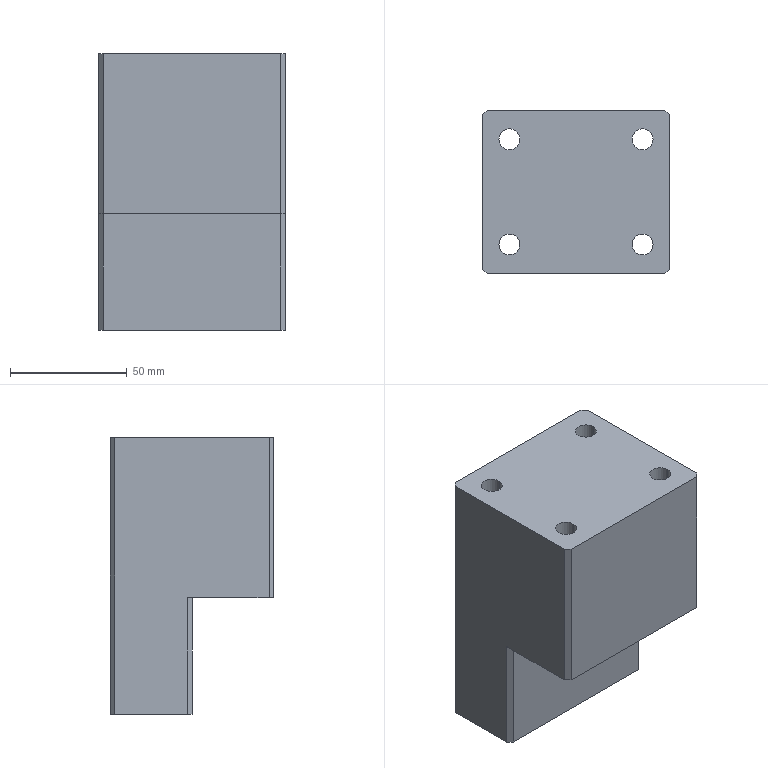Part | SolidWorks | features Cut 3, HoleWzd 2, Chamfer 1, Extrusion 1 | 1 solid | 46 faces | box 80 x 70 x 118.5 mm | volume 471238 mm3 | cylinder 22 | plane 18 | cone 6 | commonest cylinder face diameters 9 x8 14 x8 6.8 x4 14.5 x2
STEP:
#1=CARTESIAN_POINT('',(55.,50.25,6.6));
#2=VERTEX_POINT('',#1);
#3=CARTESIAN_POINT('',(55.,50.25,13.4));
#4=VERTEX_POINT('',#3);
#5=CARTESIAN_POINT('',(55.,50.25,10.));
#6=DIRECTION('',(0.,1.,0.));
#7=DIRECTION('',(0.,0.,1.));
#8=AXIS2_PLACEMENT_3D('',#5,#6,#7);
#9=CIRCLE('',#8,3.4);
#10=EDGE_CURVE('',#2,#4,#9,.T.);
#11=ORIENTED_EDGE('',*,*,#10,.F.);
#12=CARTESIAN_POINT('',(55.,70.,6.6));
#13=VERTEX_POINT('',#12);
#14=CARTESIAN_POINT('',(55.,70.,6.6));
#15=DIRECTION('',(0.,1.,0.));
#16=VECTOR('',#15,1000.);
#17=LINE('',#14,#16);
#18=EDGE_CURVE('',#2,#13,#17,.T.);
#19=ORIENTED_EDGE('',*,*,#18,.T.);
#20=CARTESIAN_POINT('',(55.,70.,13.4));
#21=VERTEX_POINT('',#20);
#22=CARTESIAN_POINT('',(55.,70.,10.));
#23=DIRECTION('',(0.,1.,0.));
#24=DIRECTION('',(0.,0.,1.));
#25=AXIS2_PLACEMENT_3D('',#22,#23,#24);
#26=CIRCLE('',#25,3.4);
#27=EDGE_CURVE('',#13,#21,#26,.T.);
#28=ORIENTED_EDGE('',*,*,#27,.T.);
#29=CARTESIAN_POINT('',(55.,70.,13.4));
#30=DIRECTION('',(0.,1.,0.));
#31=VECTOR('',#30,1000.);
#32=LINE('',#29,#31);
#33=EDGE_CURVE('',#4,#21,#32,.T.);
#34=ORIENTED_EDGE('',*,*,#33,.F.);
#35=EDGE_LOOP('',(#11,#19,#28,#34));
#36=FACE_OUTER_BOUND('',#35,.T.);
#37=CARTESIAN_POINT('',(55.,70.,10.));
#38=DIRECTION('',(0.,1.,0.));
#39=DIRECTION('',(0.,0.,1.));
#40=AXIS2_PLACEMENT_3D('',#37,#38,#39);
#41=CYLINDRICAL_SURFACE('',#40,3.4);
#42=ADVANCED_FACE('',(#36),#41,.F.);
#43=CARTESIAN_POINT('',(55.,48.207,10.));
#44=VERTEX_POINT('',#43);
#45=CARTESIAN_POINT('',(55.,50.25,13.4));
#46=DIRECTION('',(0.,0.515,0.8572));
#47=VECTOR('',#46,1000.);
#48=LINE('',#45,#47);
#49=EDGE_CURVE('',#44,#4,#48,.T.);
#50=ORIENTED_EDGE('',*,*,#49,.F.);
#51=CARTESIAN_POINT('',(55.,50.25,6.6));
#52=DIRECTION('',(0.,0.515,-0.8572));
#53=VECTOR('',#52,1000.);
#54=LINE('',#51,#53);
#55=EDGE_CURVE('',#44,#2,#54,.T.);
#56=ORIENTED_EDGE('',*,*,#55,.T.);
#57=ORIENTED_EDGE('',*,*,#10,.T.);
#58=EDGE_LOOP('',(#50,#56,#57));
#59=FACE_OUTER_BOUND('',#58,.T.);
#60=CARTESIAN_POINT('',(55.,50.25,10.));
#61=DIRECTION('',(0.,1.,0.));
#62=DIRECTION('',(0.,0.,1.));
#63=AXIS2_PLACEMENT_3D('',#60,#61,#62);
#64=CONICAL_SURFACE('',#63,3.4,1.03);
#65=ADVANCED_FACE('',(#59),#64,.F.);
#66=CARTESIAN_POINT('',(25.,50.25,6.6));
#67=VERTEX_POINT('',#66);
#68=CARTESIAN_POINT('',(25.,50.25,13.4));
#69=VERTEX_POINT('',#68);
#70=CARTESIAN_POINT('',(25.,50.25,10.));
#71=DIRECTION('',(0.,1.,0.));
#72=DIRECTION('',(0.,0.,1.));
#73=AXIS2_PLACEMENT_3D('',#70,#71,#72);
#74=CIRCLE('',#73,3.4);
#75=EDGE_CURVE('',#67,#69,#74,.T.);
#76=ORIENTED_EDGE('',*,*,#75,.F.);
#77=CARTESIAN_POINT('',(25.,70.,6.6));
#78=VERTEX_POINT('',#77);
#79=CARTESIAN_POINT('',(25.,70.,6.6));
#80=DIRECTION('',(0.,1.,0.));
#81=VECTOR('',#80,1000.);
#82=LINE('',#79,#81);
#83=EDGE_CURVE('',#67,#78,#82,.T.);
#84=ORIENTED_EDGE('',*,*,#83,.T.);
#85=CARTESIAN_POINT('',(25.,70.,13.4));
#86=VERTEX_POINT('',#85);
#87=CARTESIAN_POINT('',(25.,70.,10.));
#88=DIRECTION('',(0.,1.,0.));
#89=DIRECTION('',(0.,0.,1.));
#90=AXIS2_PLACEMENT_3D('',#87,#88,#89);
#91=CIRCLE('',#90,3.4);
#92=EDGE_CURVE('',#78,#86,#91,.T.);
#93=ORIENTED_EDGE('',*,*,#92,.T.);
#94=CARTESIAN_POINT('',(25.,70.,13.4));
#95=DIRECTION('',(0.,1.,0.));
#96=VECTOR('',#95,1000.);
#97=LINE('',#94,#96);
#98=EDGE_CURVE('',#69,#86,#97,.T.);
#99=ORIENTED_EDGE('',*,*,#98,.F.);
#100=EDGE_LOOP('',(#76,#84,#93,#99));
#101=FACE_OUTER_BOUND('',#100,.T.);
#102=CARTESIAN_POINT('',(25.,70.,10.));
#103=DIRECTION('',(0.,1.,0.));
#104=DIRECTION('',(0.,0.,1.));
#105=AXIS2_PLACEMENT_3D('',#102,#103,#104);
#106=CYLINDRICAL_SURFACE('',#105,3.4);
#107=ADVANCED_FACE('',(#101),#106,.F.);
#108=CARTESIAN_POINT('',(25.,48.207,10.));
#109=VERTEX_POINT('',#108);
#110=CARTESIAN_POINT('',(25.,50.25,13.4));
#111=DIRECTION('',(0.,0.515,0.8572));
#112=VECTOR('',#111,1000.);
#113=LINE('',#110,#112);
#114=EDGE_CURVE('',#109,#69,#113,.T.);
#115=ORIENTED_EDGE('',*,*,#114,.F.);
#116=CARTESIAN_POINT('',(25.,50.25,6.6));
#117=DIRECTION('',(0.,0.515,-0.8572));
#118=VECTOR('',#117,1000.);
#119=LINE('',#116,#118);
#120=EDGE_CURVE('',#109,#67,#119,.T.);
#121=ORIENTED_EDGE('',*,*,#120,.T.);
#122=ORIENTED_EDGE('',*,*,#75,.T.);
#123=EDGE_LOOP('',(#115,#121,#122));
#124=FACE_OUTER_BOUND('',#123,.T.);
#125=CARTESIAN_POINT('',(25.,50.25,10.));
#126=DIRECTION('',(0.,1.,0.));
#127=DIRECTION('',(0.,0.,1.));
#128=AXIS2_PLACEMENT_3D('',#125,#126,#127);
#129=CONICAL_SURFACE('',#128,3.4,1.03);
#130=ADVANCED_FACE('',(#124),#129,.F.);
#131=CARTESIAN_POINT('',(40.,33.5,90.25));
#132=VERTEX_POINT('',#131);
#133=CARTESIAN_POINT('',(40.,33.5,104.75));
#134=VERTEX_POINT('',#133);
#135=CARTESIAN_POINT('',(40.,33.5,97.5));
#136=DIRECTION('',(0.,1.,0.));
#137=DIRECTION('',(0.,0.,1.));
#138=AXIS2_PLACEMENT_3D('',#135,#136,#137);
#139=CIRCLE('',#138,7.25);
#140=EDGE_CURVE('',#132,#134,#139,.T.);
#141=ORIENTED_EDGE('',*,*,#140,.F.);
#142=CARTESIAN_POINT('',(40.,70.,90.25));
#143=VERTEX_POINT('',#142);
#144=CARTESIAN_POINT('',(40.,70.,90.25));
#145=DIRECTION('',(0.,1.,0.));
#146=VECTOR('',#145,1000.);
#147=LINE('',#144,#146);
#148=EDGE_CURVE('',#132,#143,#147,.T.);
#149=ORIENTED_EDGE('',*,*,#148,.T.);
#150=CARTESIAN_POINT('',(40.,70.,104.75));
#151=VERTEX_POINT('',#150);
#152=CARTESIAN_POINT('',(40.,70.,97.5));
#153=DIRECTION('',(0.,1.,0.));
#154=DIRECTION('',(0.,0.,1.));
#155=AXIS2_PLACEMENT_3D('',#152,#153,#154);
#156=CIRCLE('',#155,7.25);
#157=EDGE_CURVE('',#143,#151,#156,.T.);
#158=ORIENTED_EDGE('',*,*,#157,.T.);
#159=CARTESIAN_POINT('',(40.,70.,104.75));
#160=DIRECTION('',(0.,1.,0.));
#161=VECTOR('',#160,1000.);
#162=LINE('',#159,#161);
#163=EDGE_CURVE('',#134,#151,#162,.T.);
#164=ORIENTED_EDGE('',*,*,#163,.F.);
#165=EDGE_LOOP('',(#141,#149,#158,#164));
#166=FACE_OUTER_BOUND('',#165,.T.);
#167=CARTESIAN_POINT('',(40.,70.,97.5));
#168=DIRECTION('',(0.,1.,0.));
#169=DIRECTION('',(0.,0.,1.));
#170=AXIS2_PLACEMENT_3D('',#167,#168,#169);
#171=CYLINDRICAL_SURFACE('',#170,7.25);
#172=ADVANCED_FACE('',(#166),#171,.F.);
#173=CARTESIAN_POINT('',(40.,29.144,97.5));
#174=VERTEX_POINT('',#173);
#175=CARTESIAN_POINT('',(40.,33.5,104.75));
#176=DIRECTION('',(0.,0.515,0.8572));
#177=VECTOR('',#176,1000.);
#178=LINE('',#175,#177);
#179=EDGE_CURVE('',#174,#134,#178,.T.);
#180=ORIENTED_EDGE('',*,*,#179,.F.);
#181=CARTESIAN_POINT('',(40.,33.5,90.25));
#182=DIRECTION('',(0.,0.515,-0.8572));
#183=VECTOR('',#182,1000.);
#184=LINE('',#181,#183);
#185=EDGE_CURVE('',#174,#132,#184,.T.);
#186=ORIENTED_EDGE('',*,*,#185,.T.);
#187=ORIENTED_EDGE('',*,*,#140,.T.);
#188=EDGE_LOOP('',(#180,#186,#187));
#189=FACE_OUTER_BOUND('',#188,.T.);
#190=CARTESIAN_POINT('',(40.,33.5,97.5));
#191=DIRECTION('',(0.,1.,0.));
#192=DIRECTION('',(0.,0.,1.));
#193=AXIS2_PLACEMENT_3D('',#190,#191,#192);
#194=CONICAL_SURFACE('',#193,7.25,1.03);
#195=ADVANCED_FACE('',(#189),#194,.F.);
#196=CARTESIAN_POINT('',(73.,12.5,118.5));
#197=VERTEX_POINT('',#196);
#198=CARTESIAN_POINT('',(64.,12.5,118.5));
#199=VERTEX_POINT('',#198);
#200=CARTESIAN_POINT('',(68.5,12.5,118.5));
#201=DIRECTION('',(0.,0.,-1.));
#202=DIRECTION('',(-1.,0.,0.));
#203=AXIS2_PLACEMENT_3D('',#200,#201,#202);
#204=CIRCLE('',#203,4.5);
#205=EDGE_CURVE('',#197,#199,#204,.T.);
#206=ORIENTED_EDGE('',*,*,#205,.F.);
#207=CARTESIAN_POINT('',(73.,12.5,80.));
#208=VERTEX_POINT('',#207);
#209=CARTESIAN_POINT('',(73.,12.5,118.5));
#210=DIRECTION('',(0.,0.,-1.));
#211=VECTOR('',#210,1000.);
#212=LINE('',#209,#211);
#213=EDGE_CURVE('',#197,#208,#212,.T.);
#214=ORIENTED_EDGE('',*,*,#213,.T.);
#215=CARTESIAN_POINT('',(64.,12.5,80.));
#216=VERTEX_POINT('',#215);
#217=CARTESIAN_POINT('',(68.5,12.5,80.));
#218=DIRECTION('',(0.,0.,-1.));
#219=DIRECTION('',(-1.,0.,0.));
#220=AXIS2_PLACEMENT_3D('',#217,#218,#219);
#221=CIRCLE('',#220,4.5);
#222=EDGE_CURVE('',#208,#216,#221,.T.);
#223=ORIENTED_EDGE('',*,*,#222,.T.);
#224=CARTESIAN_POINT('',(64.,12.5,118.5));
#225=DIRECTION('',(0.,0.,-1.));
#226=VECTOR('',#225,1000.);
#227=LINE('',#224,#226);
#228=EDGE_CURVE('',#199,#216,#227,.T.);
#229=ORIENTED_EDGE('',*,*,#228,.F.);
#230=EDGE_LOOP('',(#206,#214,#223,#229));
#231=FACE_OUTER_BOUND('',#230,.T.);
#232=CARTESIAN_POINT('',(68.5,12.5,118.5));
#233=DIRECTION('',(0.,0.,-1.));
#234=DIRECTION('',(-1.,0.,0.));
#235=AXIS2_PLACEMENT_3D('',#232,#233,#234);
#236=CYLINDRICAL_SURFACE('',#235,4.5);
#237=ADVANCED_FACE('',(#231),#236,.F.);
#238=CARTESIAN_POINT('',(16.,12.5,118.5));
#239=VERTEX_POINT('',#238);
#240=CARTESIAN_POINT('',(7.,12.5,118.5));
#241=VERTEX_POINT('',#240);
#242=CARTESIAN_POINT('',(11.5,12.5,118.5));
#243=DIRECTION('',(0.,0.,-1.));
#244=DIRECTION('',(-1.,0.,0.));
#245=AXIS2_PLACEMENT_3D('',#242,#243,#244);
#246=CIRCLE('',#245,4.5);
#247=EDGE_CURVE('',#239,#241,#246,.T.);
#248=ORIENTED_EDGE('',*,*,#247,.F.);
#249=CARTESIAN_POINT('',(16.,12.5,80.));
#250=VERTEX_POINT('',#249);
#251=CARTESIAN_POINT('',(16.,12.5,118.5));
#252=DIRECTION('',(0.,0.,-1.));
#253=VECTOR('',#252,1000.);
#254=LINE('',#251,#253);
#255=EDGE_CURVE('',#239,#250,#254,.T.);
#256=ORIENTED_EDGE('',*,*,#255,.T.);
#257=CARTESIAN_POINT('',(7.,12.5,80.));
#258=VERTEX_POINT('',#257);
#259=CARTESIAN_POINT('',(11.5,12.5,80.));
#260=DIRECTION('',(0.,0.,-1.));
#261=DIRECTION('',(-1.,0.,0.));
#262=AXIS2_PLACEMENT_3D('',#259,#260,#261);
#263=CIRCLE('',#262,4.5);
#264=EDGE_CURVE('',#250,#258,#263,.T.);
#265=ORIENTED_EDGE('',*,*,#264,.T.);
#266=CARTESIAN_POINT('',(7.,12.5,118.5));
#267=DIRECTION('',(0.,0.,-1.));
#268=VECTOR('',#267,1000.);
#269=LINE('',#266,#268);
#270=EDGE_CURVE('',#241,#258,#269,.T.);
#271=ORIENTED_EDGE('',*,*,#270,.F.);
#272=EDGE_LOOP('',(#248,#256,#265,#271));
#273=FACE_OUTER_BOUND('',#272,.T.);
#274=CARTESIAN_POINT('',(11.5,12.5,118.5));
#275=DIRECTION('',(0.,0.,-1.));
#276=DIRECTION('',(-1.,0.,0.));
#277=AXIS2_PLACEMENT_3D('',#274,#275,#276);
#278=CYLINDRICAL_SURFACE('',#277,4.5);
#279=ADVANCED_FACE('',(#273),#278,.F.);
#280=CARTESIAN_POINT('',(16.,57.5,118.5));
#281=VERTEX_POINT('',#280);
#282=CARTESIAN_POINT('',(7.,57.5,118.5));
#283=VERTEX_POINT('',#282);
#284=CARTESIAN_POINT('',(11.5,57.5,118.5));
#285=DIRECTION('',(0.,0.,-1.));
#286=DIRECTION('',(-1.,0.,0.));
#287=AXIS2_PLACEMENT_3D('',#284,#285,#286);
#288=CIRCLE('',#287,4.5);
#289=EDGE_CURVE('',#281,#283,#288,.T.);
#290=ORIENTED_EDGE('',*,*,#289,.F.);
#291=CARTESIAN_POINT('',(16.,57.5,80.));
#292=VERTEX_POINT('',#291);
#293=CARTESIAN_POINT('',(16.,57.5,118.5));
#294=DIRECTION('',(0.,0.,-1.));
#295=VECTOR('',#294,1000.);
#296=LINE('',#293,#295);
#297=EDGE_CURVE('',#281,#292,#296,.T.);
#298=ORIENTED_EDGE('',*,*,#297,.T.);
#299=CARTESIAN_POINT('',(7.,57.5,80.));
#300=VERTEX_POINT('',#299);
#301=CARTESIAN_POINT('',(11.5,57.5,80.));
#302=DIRECTION('',(0.,0.,-1.));
#303=DIRECTION('',(-1.,0.,0.));
#304=AXIS2_PLACEMENT_3D('',#301,#302,#303);
#305=CIRCLE('',#304,4.5);
#306=EDGE_CURVE('',#292,#300,#305,.T.);
#307=ORIENTED_EDGE('',*,*,#306,.T.);
#308=CARTESIAN_POINT('',(7.,57.5,118.5));
#309=DIRECTION('',(0.,0.,-1.));
#310=VECTOR('',#309,1000.);
#311=LINE('',#308,#310);
#312=EDGE_CURVE('',#283,#300,#311,.T.);
#313=ORIENTED_EDGE('',*,*,#312,.F.);
#314=EDGE_LOOP('',(#290,#298,#307,#313));
#315=FACE_OUTER_BOUND('',#314,.T.);
#316=CARTESIAN_POINT('',(11.5,57.5,118.5));
#317=DIRECTION('',(0.,0.,-1.));
#318=DIRECTION('',(-1.,0.,0.));
#319=AXIS2_PLACEMENT_3D('',#316,#317,#318);
#320=CYLINDRICAL_SURFACE('',#319,4.5);
#321=ADVANCED_FACE('',(#315),#320,.F.);
#322=CARTESIAN_POINT('',(73.,57.5,118.5));
#323=VERTEX_POINT('',#322);
#324=CARTESIAN_POINT('',(64.,57.5,118.5));
#325=VERTEX_POINT('',#324);
#326=CARTESIAN_POINT('',(68.5,57.5,118.5));
#327=DIRECTION('',(0.,0.,-1.));
#328=DIRECTION('',(-1.,0.,0.));
#329=AXIS2_PLACEMENT_3D('',#326,#327,#328);
#330=CIRCLE('',#329,4.5);
#331=EDGE_CURVE('',#323,#325,#330,.T.);
#332=ORIENTED_EDGE('',*,*,#331,.F.);
#333=CARTESIAN_POINT('',(73.,57.5,80.));
#334=VERTEX_POINT('',#333);
#335=CARTESIAN_POINT('',(73.,57.5,118.5));
#336=DIRECTION('',(0.,0.,-1.));
#337=VECTOR('',#336,1000.);
#338=LINE('',#335,#337);
#339=EDGE_CURVE('',#323,#334,#338,.T.);
#340=ORIENTED_EDGE('',*,*,#339,.T.);
#341=CARTESIAN_POINT('',(64.,57.5,80.));
#342=VERTEX_POINT('',#341);
#343=CARTESIAN_POINT('',(68.5,57.5,80.));
#344=DIRECTION('',(0.,0.,-1.));
#345=DIRECTION('',(-1.,0.,0.));
#346=AXIS2_PLACEMENT_3D('',#343,#344,#345);
#347=CIRCLE('',#346,4.5);
#348=EDGE_CURVE('',#334,#342,#347,.T.);
#349=ORIENTED_EDGE('',*,*,#348,.T.);
#350=CARTESIAN_POINT('',(64.,57.5,118.5));
#351=DIRECTION('',(0.,0.,-1.));
#352=VECTOR('',#351,1000.);
#353=LINE('',#350,#352);
#354=EDGE_CURVE('',#325,#342,#353,.T.);
#355=ORIENTED_EDGE('',*,*,#354,.F.);
#356=EDGE_LOOP('',(#332,#340,#349,#355));
#357=FACE_OUTER_BOUND('',#356,.T.);
#358=CARTESIAN_POINT('',(68.5,57.5,118.5));
#359=DIRECTION('',(0.,0.,-1.));
#360=DIRECTION('',(-1.,0.,0.));
#361=AXIS2_PLACEMENT_3D('',#358,#359,#360);
#362=CYLINDRICAL_SURFACE('',#361,4.5);
#363=ADVANCED_FACE('',(#357),#362,.F.);
#364=CARTESIAN_POINT('',(75.5,12.5,80.));
#365=VERTEX_POINT('',#364);
#366=CARTESIAN_POINT('',(61.5,12.5,80.));
#367=VERTEX_POINT('',#366);
#368=CARTESIAN_POINT('',(68.5,12.5,80.));
#369=DIRECTION('',(0.,0.,-1.));
#370=DIRECTION('',(-1.,0.,0.));
#371=AXIS2_PLACEMENT_3D('',#368,#369,#370);
#372=CIRCLE('',#371,7.);
#373=EDGE_CURVE('',#365,#367,#372,.T.);
#374=ORIENTED_EDGE('',*,*,#373,.F.);
#375=CARTESIAN_POINT('',(75.5,12.5,50.));
#376=VERTEX_POINT('',#375);
#377=CARTESIAN_POINT('',(75.5,12.5,80.));
#378=DIRECTION('',(0.,0.,-1.));
#379=VECTOR('',#378,1000.);
#380=LINE('',#377,#379);
#381=EDGE_CURVE('',#365,#376,#380,.T.);
#382=ORIENTED_EDGE('',*,*,#381,.T.);
#383=CARTESIAN_POINT('',(61.5,12.5,50.));
#384=VERTEX_POINT('',#383);
#385=CARTESIAN_POINT('',(68.5,12.5,50.));
#386=DIRECTION('',(0.,0.,-1.));
#387=DIRECTION('',(1.,0.,0.));
#388=AXIS2_PLACEMENT_3D('',#385,#386,#387);
#389=CIRCLE('',#388,7.);
#390=EDGE_CURVE('',#376,#384,#389,.T.);
#391=ORIENTED_EDGE('',*,*,#390,.T.);
#392=CARTESIAN_POINT('',(61.5,12.5,80.));
#393=DIRECTION('',(0.,0.,-1.));
#394=VECTOR('',#393,1000.);
#395=LINE('',#392,#394);
#396=EDGE_CURVE('',#367,#384,#395,.T.);
#397=ORIENTED_EDGE('',*,*,#396,.F.);
#398=EDGE_LOOP('',(#374,#382,#391,#397));
#399=FACE_OUTER_BOUND('',#398,.T.);
#400=CARTESIAN_POINT('',(68.5,12.5,80.));
#401=DIRECTION('',(0.,0.,-1.));
#402=DIRECTION('',(-1.,0.,0.));
#403=AXIS2_PLACEMENT_3D('',#400,#401,#402);
#404=CYLINDRICAL_SURFACE('',#403,7.);
#405=ADVANCED_FACE('',(#399),#404,.F.);
#406=CARTESIAN_POINT('',(75.5,57.5,80.));
#407=VERTEX_POINT('',#406);
#408=CARTESIAN_POINT('',(61.5,57.5,80.));
#409=VERTEX_POINT('',#408);
#410=CARTESIAN_POINT('',(68.5,57.5,80.));
#411=DIRECTION('',(0.,0.,-1.));
#412=DIRECTION('',(-1.,0.,0.));
#413=AXIS2_PLACEMENT_3D('',#410,#411,#412);
#414=CIRCLE('',#413,7.);
#415=EDGE_CURVE('',#407,#409,#414,.T.);
#416=ORIENTED_EDGE('',*,*,#415,.F.);
#417=CARTESIAN_POINT('',(75.5,57.5,0.));
#418=VERTEX_POINT('',#417);
#419=CARTESIAN_POINT('',(75.5,57.5,80.));
#420=DIRECTION('',(0.,0.,-1.));
#421=VECTOR('',#420,1000.);
#422=LINE('',#419,#421);
#423=EDGE_CURVE('',#407,#418,#422,.T.);
#424=ORIENTED_EDGE('',*,*,#423,.T.);
#425=CARTESIAN_POINT('',(61.5,57.5,0.));
#426=VERTEX_POINT('',#425);
#427=CARTESIAN_POINT('',(68.5,57.5,0.));
#428=DIRECTION('',(0.,0.,-1.));
#429=DIRECTION('',(-1.,0.,0.));
#430=AXIS2_PLACEMENT_3D('',#427,#428,#429);
#431=CIRCLE('',#430,7.);
#432=EDGE_CURVE('',#418,#426,#431,.T.);
#433=ORIENTED_EDGE('',*,*,#432,.T.);
#434=CARTESIAN_POINT('',(61.5,57.5,80.));
#435=DIRECTION('',(0.,0.,-1.));
#436=VECTOR('',#435,1000.);
#437=LINE('',#434,#436);
#438=EDGE_CURVE('',#409,#426,#437,.T.);
#439=ORIENTED_EDGE('',*,*,#438,.F.);
#440=EDGE_LOOP('',(#416,#424,#433,#439));
#441=FACE_OUTER_BOUND('',#440,.T.);
#442=CARTESIAN_POINT('',(68.5,57.5,80.));
#443=DIRECTION('',(0.,0.,-1.));
#444=DIRECTION('',(-1.,0.,0.));
#445=AXIS2_PLACEMENT_3D('',#442,#443,#444);
#446=CYLINDRICAL_SURFACE('',#445,7.);
#447=ADVANCED_FACE('',(#441),#446,.F.);
#448=CARTESIAN_POINT('',(18.5,12.5,80.));
#449=VERTEX_POINT('',#448);
#450=CARTESIAN_POINT('',(4.5,12.5,80.));
#451=VERTEX_POINT('',#450);
#452=CARTESIAN_POINT('',(11.5,12.5,80.));
#453=DIRECTION('',(0.,0.,-1.));
#454=DIRECTION('',(-1.,0.,0.));
#455=AXIS2_PLACEMENT_3D('',#452,#453,#454);
#456=CIRCLE('',#455,7.);
#457=EDGE_CURVE('',#449,#451,#456,.T.);
#458=ORIENTED_EDGE('',*,*,#457,.F.);
#459=CARTESIAN_POINT('',(18.5,12.5,50.));
#460=VERTEX_POINT('',#459);
#461=CARTESIAN_POINT('',(18.5,12.5,80.));
#462=DIRECTION('',(0.,0.,-1.));
#463=VECTOR('',#462,1000.);
#464=LINE('',#461,#463);
#465=EDGE_CURVE('',#449,#460,#464,.T.);
#466=ORIENTED_EDGE('',*,*,#465,.T.);
#467=CARTESIAN_POINT('',(4.5,12.5,50.));
#468=VERTEX_POINT('',#467);
#469=CARTESIAN_POINT('',(11.5,12.5,50.));
#470=DIRECTION('',(0.,0.,-1.));
#471=DIRECTION('',(1.,0.,0.));
#472=AXIS2_PLACEMENT_3D('',#469,#470,#471);
#473=CIRCLE('',#472,7.);
#474=EDGE_CURVE('',#460,#468,#473,.T.);
#475=ORIENTED_EDGE('',*,*,#474,.T.);
#476=CARTESIAN_POINT('',(4.5,12.5,80.));
#477=DIRECTION('',(0.,0.,-1.));
#478=VECTOR('',#477,1000.);
#479=LINE('',#476,#478);
#480=EDGE_CURVE('',#451,#468,#479,.T.);
#481=ORIENTED_EDGE('',*,*,#480,.F.);
#482=EDGE_LOOP('',(#458,#466,#475,#481));
#483=FACE_OUTER_BOUND('',#482,.T.);
#484=CARTESIAN_POINT('',(11.5,12.5,80.));
#485=DIRECTION('',(0.,0.,-1.));
#486=DIRECTION('',(-1.,0.,0.));
#487=AXIS2_PLACEMENT_3D('',#484,#485,#486);
#488=CYLINDRICAL_SURFACE('',#487,7.);
#489=ADVANCED_FACE('',(#483),#488,.F.);
#490=CARTESIAN_POINT('',(18.5,57.5,80.));
#491=VERTEX_POINT('',#490);
#492=CARTESIAN_POINT('',(4.5,57.5,80.));
#493=VERTEX_POINT('',#492);
#494=CARTESIAN_POINT('',(11.5,57.5,80.));
#495=DIRECTION('',(0.,0.,-1.));
#496=DIRECTION('',(-1.,0.,0.));
#497=AXIS2_PLACEMENT_3D('',#494,#495,#496);
#498=CIRCLE('',#497,7.);
#499=EDGE_CURVE('',#491,#493,#498,.T.);
#500=ORIENTED_EDGE('',*,*,#499,.F.);
#501=CARTESIAN_POINT('',(18.5,57.5,0.));
#502=VERTEX_POINT('',#501);
#503=CARTESIAN_POINT('',(18.5,57.5,80.));
#504=DIRECTION('',(0.,0.,-1.));
#505=VECTOR('',#504,1000.);
#506=LINE('',#503,#505);
#507=EDGE_CURVE('',#491,#502,#506,.T.);
#508=ORIENTED_EDGE('',*,*,#507,.T.);
#509=CARTESIAN_POINT('',(4.5,57.5,0.));
#510=VERTEX_POINT('',#509);
#511=CARTESIAN_POINT('',(11.5,57.5,0.));
#512=DIRECTION('',(0.,0.,-1.));
#513=DIRECTION('',(-1.,0.,0.));
#514=AXIS2_PLACEMENT_3D('',#511,#512,#513);
#515=CIRCLE('',#514,7.);
#516=EDGE_CURVE('',#502,#510,#515,.T.);
#517=ORIENTED_EDGE('',*,*,#516,.T.);
#518=CARTESIAN_POINT('',(4.5,57.5,80.));
#519=DIRECTION('',(0.,0.,-1.));
#520=VECTOR('',#519,1000.);
#521=LINE('',#518,#520);
#522=EDGE_CURVE('',#493,#510,#521,.T.);
#523=ORIENTED_EDGE('',*,*,#522,.F.);
#524=EDGE_LOOP('',(#500,#508,#517,#523));
#525=FACE_OUTER_BOUND('',#524,.T.);
#526=CARTESIAN_POINT('',(11.5,57.5,80.));
#527=DIRECTION('',(0.,0.,-1.));
#528=DIRECTION('',(-1.,0.,0.));
#529=AXIS2_PLACEMENT_3D('',#526,#527,#528);
#530=CYLINDRICAL_SURFACE('',#529,7.);
#531=ADVANCED_FACE('',(#525),#530,.F.);
#532=CARTESIAN_POINT('',(0.,68.,0.));
#533=VERTEX_POINT('',#532);
#534=CARTESIAN_POINT('',(0.,37.,0.));
#535=VERTEX_POINT('',#534);
#536=CARTESIAN_POINT('',(0.,0.,0.));
#537=DIRECTION('',(0.,-1.,0.));
#538=VECTOR('',#537,1000.);
#539=LINE('',#536,#538);
#540=EDGE_CURVE('',#533,#535,#539,.T.);
#541=ORIENTED_EDGE('',*,*,#540,.T.);
#542=CARTESIAN_POINT('',(0.,37.,50.));
#543=VERTEX_POINT('',#542);
#544=CARTESIAN_POINT('',(0.,37.,118.5));
#545=DIRECTION('',(0.,0.,1.));
#546=VECTOR('',#545,1000.);
#547=LINE('',#544,#546);
#548=EDGE_CURVE('',#535,#543,#547,.T.);
#549=ORIENTED_EDGE('',*,*,#548,.T.);
#550=CARTESIAN_POINT('',(0.,2.,50.));
#551=VERTEX_POINT('',#550);
#552=CARTESIAN_POINT('',(0.,0.,50.));
#553=DIRECTION('',(0.,1.,0.));
#554=VECTOR('',#553,1000.);
#555=LINE('',#552,#554);
#556=EDGE_CURVE('',#551,#543,#555,.T.);
#557=ORIENTED_EDGE('',*,*,#556,.F.);
#558=CARTESIAN_POINT('',(0.,2.,118.5));
#559=VERTEX_POINT('',#558);
#560=CARTESIAN_POINT('',(0.,2.,118.5));
#561=DIRECTION('',(0.,0.,1.));
#562=VECTOR('',#561,1000.);
#563=LINE('',#560,#562);
#564=EDGE_CURVE('',#551,#559,#563,.T.);
#565=ORIENTED_EDGE('',*,*,#564,.T.);
#566=CARTESIAN_POINT('',(0.,68.,118.5));
#567=VERTEX_POINT('',#566);
#568=CARTESIAN_POINT('',(0.,0.,118.5));
#569=DIRECTION('',(0.,-1.,0.));
#570=VECTOR('',#569,1000.);
#571=LINE('',#568,#570);
#572=EDGE_CURVE('',#567,#559,#571,.T.);
#573=ORIENTED_EDGE('',*,*,#572,.F.);
#574=CARTESIAN_POINT('',(0.,68.,118.5));
#575=DIRECTION('',(0.,0.,-1.));
#576=VECTOR('',#575,1000.);
#577=LINE('',#574,#576);
#578=EDGE_CURVE('',#567,#533,#577,.T.);
#579=ORIENTED_EDGE('',*,*,#578,.T.);
#580=EDGE_LOOP('',(#541,#549,#557,#565,#573,#579));
#581=FACE_OUTER_BOUND('',#580,.T.);
#582=CARTESIAN_POINT('',(0.,0.,118.5));
#583=DIRECTION('',(1.,0.,0.));
#584=DIRECTION('',(0.,1.,0.));
#585=AXIS2_PLACEMENT_3D('',#582,#583,#584);
#586=PLANE('',#585);
#587=ADVANCED_FACE('',(#581),#586,.F.);
#588=CARTESIAN_POINT('',(2.,0.,118.5));
#589=VERTEX_POINT('',#588);
#590=CARTESIAN_POINT('',(78.,0.,118.5));
#591=VERTEX_POINT('',#590);
#592=CARTESIAN_POINT('',(0.,0.,118.5));
#593=DIRECTION('',(1.,0.,0.));
#594=VECTOR('',#593,1000.);
#595=LINE('',#592,#594);
#596=EDGE_CURVE('',#589,#591,#595,.T.);
#597=ORIENTED_EDGE('',*,*,#596,.F.);
#598=CARTESIAN_POINT('',(2.,0.,50.));
#599=VERTEX_POINT('',#598);
#600=CARTESIAN_POINT('',(2.,0.,118.5));
#601=DIRECTION('',(0.,0.,-1.));
#602=VECTOR('',#601,1000.);
#603=LINE('',#600,#602);
#604=EDGE_CURVE('',#589,#599,#603,.T.);
#605=ORIENTED_EDGE('',*,*,#604,.T.);
#606=CARTESIAN_POINT('',(78.,0.,50.));
#607=VERTEX_POINT('',#606);
#608=CARTESIAN_POINT('',(80.,0.,50.));
#609=DIRECTION('',(-1.,0.,0.));
#610=VECTOR('',#609,1000.);
#611=LINE('',#608,#610);
#612=EDGE_CURVE('',#607,#599,#611,.T.);
#613=ORIENTED_EDGE('',*,*,#612,.F.);
#614=CARTESIAN_POINT('',(78.,0.,118.5));
#615=DIRECTION('',(0.,0.,1.));
#616=VECTOR('',#615,1000.);
#617=LINE('',#614,#616);
#618=EDGE_CURVE('',#607,#591,#617,.T.);
#619=ORIENTED_EDGE('',*,*,#618,.T.);
#620=EDGE_LOOP('',(#597,#605,#613,#619));
#621=FACE_OUTER_BOUND('',#620,.T.);
#622=CARTESIAN_POINT('',(0.,0.,118.5));
#623=DIRECTION('',(0.,1.,0.));
#624=DIRECTION('',(0.,0.,1.));
#625=AXIS2_PLACEMENT_3D('',#622,#623,#624);
#626=PLANE('',#625);
#627=ADVANCED_FACE('',(#621),#626,.F.);
#628=CARTESIAN_POINT('',(80.,37.,50.));
#629=VERTEX_POINT('',#628);
#630=CARTESIAN_POINT('',(80.,2.,50.));
#631=VERTEX_POINT('',#630);
#632=CARTESIAN_POINT('',(80.,0.,50.));
#633=DIRECTION('',(0.,-1.,0.));
#634=VECTOR('',#633,1000.);
#635=LINE('',#632,#634);
#636=EDGE_CURVE('',#629,#631,#635,.T.);
#637=ORIENTED_EDGE('',*,*,#636,.F.);
#638=CARTESIAN_POINT('',(80.,37.,0.));
#639=VERTEX_POINT('',#638);
#640=CARTESIAN_POINT('',(80.,37.,118.5));
#641=DIRECTION('',(0.,0.,-1.));
#642=VECTOR('',#641,1000.);
#643=LINE('',#640,#642);
#644=EDGE_CURVE('',#629,#639,#643,.T.);
#645=ORIENTED_EDGE('',*,*,#644,.T.);
#646=CARTESIAN_POINT('',(80.,68.,0.));
#647=VERTEX_POINT('',#646);
#648=CARTESIAN_POINT('',(80.,0.,0.));
#649=DIRECTION('',(0.,1.,0.));
#650=VECTOR('',#649,1000.);
#651=LINE('',#648,#650);
#652=EDGE_CURVE('',#639,#647,#651,.T.);
#653=ORIENTED_EDGE('',*,*,#652,.T.);
#654=CARTESIAN_POINT('',(80.,68.,118.5));
#655=VERTEX_POINT('',#654);
#656=CARTESIAN_POINT('',(80.,68.,118.5));
#657=DIRECTION('',(0.,0.,1.));
#658=VECTOR('',#657,1000.);
#659=LINE('',#656,#658);
#660=EDGE_CURVE('',#647,#655,#659,.T.);
#661=ORIENTED_EDGE('',*,*,#660,.T.);
#662=CARTESIAN_POINT('',(80.,2.,118.5));
#663=VERTEX_POINT('',#662);
#664=CARTESIAN_POINT('',(80.,0.,118.5));
#665=DIRECTION('',(0.,1.,0.));
#666=VECTOR('',#665,1000.);
#667=LINE('',#664,#666);
#668=EDGE_CURVE('',#663,#655,#667,.T.);
#669=ORIENTED_EDGE('',*,*,#668,.F.);
#670=CARTESIAN_POINT('',(80.,2.,118.5));
#671=DIRECTION('',(0.,0.,-1.));
#672=VECTOR('',#671,1000.);
#673=LINE('',#670,#672);
#674=EDGE_CURVE('',#663,#631,#673,.T.);
#675=ORIENTED_EDGE('',*,*,#674,.T.);
#676=EDGE_LOOP('',(#637,#645,#653,#661,#669,#675));
#677=FACE_OUTER_BOUND('',#676,.T.);
#678=CARTESIAN_POINT('',(80.,0.,118.5));
#679=DIRECTION('',(-1.,0.,0.));
#680=DIRECTION('',(0.,-1.,0.));
#681=AXIS2_PLACEMENT_3D('',#678,#679,#680);
#682=PLANE('',#681);
#683=ADVANCED_FACE('',(#677),#682,.F.);
#684=CARTESIAN_POINT('',(55.,70.,10.));
#685=DIRECTION('',(0.,1.,0.));
#686=DIRECTION('',(0.,0.,1.));
#687=AXIS2_PLACEMENT_3D('',#684,#685,#686);
#688=CIRCLE('',#687,3.4);
#689=EDGE_CURVE('',#21,#13,#688,.T.);
#690=ORIENTED_EDGE('',*,*,#689,.F.);
#691=ORIENTED_EDGE('',*,*,#27,.F.);
#692=EDGE_LOOP('',(#690,#691));
#693=FACE_BOUND('',#692,.T.);
#694=CARTESIAN_POINT('',(25.,70.,10.));
#695=DIRECTION('',(0.,1.,0.));
#696=DIRECTION('',(0.,0.,1.));
#697=AXIS2_PLACEMENT_3D('',#694,#695,#696);
#698=CIRCLE('',#697,3.4);
#699=EDGE_CURVE('',#86,#78,#698,.T.);
#700=ORIENTED_EDGE('',*,*,#699,.F.);
#701=ORIENTED_EDGE('',*,*,#92,.F.);
#702=EDGE_LOOP('',(#700,#701));
#703=FACE_BOUND('',#702,.T.);
#704=CARTESIAN_POINT('',(40.,70.,97.5));
#705=DIRECTION('',(0.,1.,0.));
#706=DIRECTION('',(0.,0.,1.));
#707=AXIS2_PLACEMENT_3D('',#704,#705,#706);
#708=CIRCLE('',#707,7.25);
#709=EDGE_CURVE('',#151,#143,#708,.T.);
#710=ORIENTED_EDGE('',*,*,#709,.F.);
#711=ORIENTED_EDGE('',*,*,#157,.F.);
#712=EDGE_LOOP('',(#710,#711));
#713=FACE_BOUND('',#712,.T.);
#714=CARTESIAN_POINT('',(78.,70.,0.));
#715=VERTEX_POINT('',#714);
#716=CARTESIAN_POINT('',(2.,70.,0.));
#717=VERTEX_POINT('',#716);
#718=CARTESIAN_POINT('',(0.,70.,0.));
#719=DIRECTION('',(-1.,0.,0.));
#720=VECTOR('',#719,1000.);
#721=LINE('',#718,#720);
#722=EDGE_CURVE('',#715,#717,#721,.T.);
#723=ORIENTED_EDGE('',*,*,#722,.T.);
#724=CARTESIAN_POINT('',(2.,70.,118.5));
#725=VERTEX_POINT('',#724);
#726=CARTESIAN_POINT('',(2.,70.,118.5));
#727=DIRECTION('',(0.,0.,1.));
#728=VECTOR('',#727,1000.);
#729=LINE('',#726,#728);
#730=EDGE_CURVE('',#717,#725,#729,.T.);
#731=ORIENTED_EDGE('',*,*,#730,.T.);
#732=CARTESIAN_POINT('',(78.,70.,118.5));
#733=VERTEX_POINT('',#732);
#734=CARTESIAN_POINT('',(0.,70.,118.5));
#735=DIRECTION('',(-1.,0.,0.));
#736=VECTOR('',#735,1000.);
#737=LINE('',#734,#736);
#738=EDGE_CURVE('',#733,#725,#737,.T.);
#739=ORIENTED_EDGE('',*,*,#738,.F.);
#740=CARTESIAN_POINT('',(78.,70.,118.5));
#741=DIRECTION('',(0.,0.,-1.));
#742=VECTOR('',#741,1000.);
#743=LINE('',#740,#742);
#744=EDGE_CURVE('',#733,#715,#743,.T.);
#745=ORIENTED_EDGE('',*,*,#744,.T.);
#746=EDGE_LOOP('',(#723,#731,#739,#745));
#747=FACE_OUTER_BOUND('',#746,.T.);
#748=CARTESIAN_POINT('',(0.,70.,118.5));
#749=DIRECTION('',(0.,-1.,0.));
#750=DIRECTION('',(0.,0.,-1.));
#751=AXIS2_PLACEMENT_3D('',#748,#749,#750);
#752=PLANE('',#751);
#753=ADVANCED_FACE('',(#693,#703,#713,#747),#752,.F.);
#754=CARTESIAN_POINT('',(68.5,12.5,118.5));
#755=DIRECTION('',(0.,0.,-1.));
#756=DIRECTION('',(-1.,0.,0.));
#757=AXIS2_PLACEMENT_3D('',#754,#755,#756);
#758=CIRCLE('',#757,4.5);
#759=EDGE_CURVE('',#199,#197,#758,.T.);
#760=ORIENTED_EDGE('',*,*,#759,.T.);
#761=ORIENTED_EDGE('',*,*,#205,.T.);
#762=EDGE_LOOP('',(#760,#761));
#763=FACE_BOUND('',#762,.T.);
#764=CARTESIAN_POINT('',(11.5,12.5,118.5));
#765=DIRECTION('',(0.,0.,-1.));
#766=DIRECTION('',(-1.,0.,0.));
#767=AXIS2_PLACEMENT_3D('',#764,#765,#766);
#768=CIRCLE('',#767,4.5);
#769=EDGE_CURVE('',#241,#239,#768,.T.);
#770=ORIENTED_EDGE('',*,*,#769,.T.);
#771=ORIENTED_EDGE('',*,*,#247,.T.);
#772=EDGE_LOOP('',(#770,#771));
#773=FACE_BOUND('',#772,.T.);
#774=CARTESIAN_POINT('',(11.5,57.5,118.5));
#775=DIRECTION('',(0.,0.,-1.));
#776=DIRECTION('',(-1.,0.,0.));
#777=AXIS2_PLACEMENT_3D('',#774,#775,#776);
#778=CIRCLE('',#777,4.5);
#779=EDGE_CURVE('',#283,#281,#778,.T.);
#780=ORIENTED_EDGE('',*,*,#779,.T.);
#781=ORIENTED_EDGE('',*,*,#289,.T.);
#782=EDGE_LOOP('',(#780,#781));
#783=FACE_BOUND('',#782,.T.);
#784=CARTESIAN_POINT('',(68.5,57.5,118.5));
#785=DIRECTION('',(0.,0.,-1.));
#786=DIRECTION('',(-1.,0.,0.));
#787=AXIS2_PLACEMENT_3D('',#784,#785,#786);
#788=CIRCLE('',#787,4.5);
#789=EDGE_CURVE('',#325,#323,#788,.T.);
#790=ORIENTED_EDGE('',*,*,#789,.T.);
#791=ORIENTED_EDGE('',*,*,#331,.T.);
#792=EDGE_LOOP('',(#790,#791));
#793=FACE_BOUND('',#792,.T.);
#794=ORIENTED_EDGE('',*,*,#738,.T.);
#795=CARTESIAN_POINT('',(0.,68.,118.5));
#796=DIRECTION('',(-0.7071,-0.7071,0.));
#797=VECTOR('',#796,1000.);
#798=LINE('',#795,#797);
#799=EDGE_CURVE('',#725,#567,#798,.T.);
#800=ORIENTED_EDGE('',*,*,#799,.T.);
#801=ORIENTED_EDGE('',*,*,#572,.T.);
#802=CARTESIAN_POINT('',(2.,0.,118.5));
#803=DIRECTION('',(0.7071,-0.7071,0.));
#804=VECTOR('',#803,1000.);
#805=LINE('',#802,#804);
#806=EDGE_CURVE('',#559,#589,#805,.T.);
#807=ORIENTED_EDGE('',*,*,#806,.T.);
#808=ORIENTED_EDGE('',*,*,#596,.T.);
#809=CARTESIAN_POINT('',(80.,2.,118.5));
#810=DIRECTION('',(0.7071,0.7071,0.));
#811=VECTOR('',#810,1000.);
#812=LINE('',#809,#811);
#813=EDGE_CURVE('',#591,#663,#812,.T.);
#814=ORIENTED_EDGE('',*,*,#813,.T.);
#815=ORIENTED_EDGE('',*,*,#668,.T.);
#816=CARTESIAN_POINT('',(78.,70.,118.5));
#817=DIRECTION('',(-0.7071,0.7071,0.));
#818=VECTOR('',#817,1000.);
#819=LINE('',#816,#818);
#820=EDGE_CURVE('',#655,#733,#819,.T.);
#821=ORIENTED_EDGE('',*,*,#820,.T.);
#822=EDGE_LOOP('',(#794,#800,#801,#807,#808,#814,#815,#821));
#823=FACE_OUTER_BOUND('',#822,.T.);
#824=CARTESIAN_POINT('',(0.,0.,118.5));
#825=DIRECTION('',(0.,0.,-1.));
#826=DIRECTION('',(-1.,0.,0.));
#827=AXIS2_PLACEMENT_3D('',#824,#825,#826);
#828=PLANE('',#827);
#829=ADVANCED_FACE('',(#763,#773,#783,#793,#823),#828,.F.);
#830=CARTESIAN_POINT('',(2.,35.,0.));
#831=VERTEX_POINT('',#830);
#832=CARTESIAN_POINT('',(78.,35.,0.));
#833=VERTEX_POINT('',#832);
#834=CARTESIAN_POINT('',(80.,35.,0.));
#835=DIRECTION('',(1.,0.,0.));
#836=VECTOR('',#835,1000.);
#837=LINE('',#834,#836);
#838=EDGE_CURVE('',#831,#833,#837,.T.);
#839=ORIENTED_EDGE('',*,*,#838,.F.);
#840=CARTESIAN_POINT('',(18.5,18.5,0.));
#841=DIRECTION('',(-0.7071,0.7071,0.));
#842=VECTOR('',#841,1000.);
#843=LINE('',#840,#842);
#844=EDGE_CURVE('',#831,#535,#843,.T.);
#845=ORIENTED_EDGE('',*,*,#844,.T.);
#846=ORIENTED_EDGE('',*,*,#540,.F.);
#847=CARTESIAN_POINT('',(-34.,34.,0.));
#848=DIRECTION('',(0.7071,0.7071,0.));
#849=VECTOR('',#848,1000.);
#850=LINE('',#847,#849);
#851=EDGE_CURVE('',#533,#717,#850,.T.);
#852=ORIENTED_EDGE('',*,*,#851,.T.);
#853=ORIENTED_EDGE('',*,*,#722,.F.);
#854=CARTESIAN_POINT('',(74.,74.,0.));
#855=DIRECTION('',(0.7071,-0.7071,0.));
#856=VECTOR('',#855,1000.);
#857=LINE('',#854,#856);
#858=EDGE_CURVE('',#715,#647,#857,.T.);
#859=ORIENTED_EDGE('',*,*,#858,.T.);
#860=ORIENTED_EDGE('',*,*,#652,.F.);
#861=CARTESIAN_POINT('',(21.5,-21.5,0.));
#862=DIRECTION('',(-0.7071,-0.7071,0.));
#863=VECTOR('',#862,1000.);
#864=LINE('',#861,#863);
#865=EDGE_CURVE('',#639,#833,#864,.T.);
#866=ORIENTED_EDGE('',*,*,#865,.T.);
#867=EDGE_LOOP('',(#839,#845,#846,#852,#853,#859,#860,#866));
#868=FACE_OUTER_BOUND('',#867,.T.);
#869=CARTESIAN_POINT('',(68.5,57.5,0.));
#870=DIRECTION('',(0.,0.,-1.));
#871=DIRECTION('',(-1.,0.,0.));
#872=AXIS2_PLACEMENT_3D('',#869,#870,#871);
#873=CIRCLE('',#872,7.);
#874=EDGE_CURVE('',#426,#418,#873,.T.);
#875=ORIENTED_EDGE('',*,*,#874,.F.);
#876=ORIENTED_EDGE('',*,*,#432,.F.);
#877=EDGE_LOOP('',(#875,#876));
#878=FACE_BOUND('',#877,.T.);
#879=CARTESIAN_POINT('',(11.5,57.5,0.));
#880=DIRECTION('',(0.,0.,-1.));
#881=DIRECTION('',(-1.,0.,0.));
#882=AXIS2_PLACEMENT_3D('',#879,#880,#881);
#883=CIRCLE('',#882,7.);
#884=EDGE_CURVE('',#510,#502,#883,.T.);
#885=ORIENTED_EDGE('',*,*,#884,.F.);
#886=ORIENTED_EDGE('',*,*,#516,.F.);
#887=EDGE_LOOP('',(#885,#886));
#888=FACE_BOUND('',#887,.T.);
#889=CARTESIAN_POINT('',(0.,0.,0.));
#890=DIRECTION('',(0.,0.,-1.));
#891=DIRECTION('',(-1.,0.,0.));
#892=AXIS2_PLACEMENT_3D('',#889,#890,#891);
#893=PLANE('',#892);
#894=ADVANCED_FACE('',(#868,#878,#888),#893,.T.);
#895=ORIENTED_EDGE('',*,*,#507,.F.);
#896=CARTESIAN_POINT('',(11.5,57.5,80.));
#897=DIRECTION('',(0.,0.,-1.));
#898=DIRECTION('',(-1.,0.,0.));
#899=AXIS2_PLACEMENT_3D('',#896,#897,#898);
#900=CIRCLE('',#899,7.);
#901=EDGE_CURVE('',#493,#491,#900,.T.);
#902=ORIENTED_EDGE('',*,*,#901,.F.);
#903=ORIENTED_EDGE('',*,*,#522,.T.);
#904=ORIENTED_EDGE('',*,*,#884,.T.);
#905=EDGE_LOOP('',(#895,#902,#903,#904));
#906=FACE_OUTER_BOUND('',#905,.T.);
#907=CARTESIAN_POINT('',(11.5,57.5,80.));
#908=DIRECTION('',(0.,0.,-1.));
#909=DIRECTION('',(-1.,0.,0.));
#910=AXIS2_PLACEMENT_3D('',#907,#908,#909);
#911=CYLINDRICAL_SURFACE('',#910,7.);
#912=ADVANCED_FACE('',(#906),#911,.F.);
#913=CARTESIAN_POINT('',(11.5,57.5,80.));
#914=DIRECTION('',(0.,0.,-1.));
#915=DIRECTION('',(-1.,0.,0.));
#916=AXIS2_PLACEMENT_3D('',#913,#914,#915);
#917=CIRCLE('',#916,4.5);
#918=EDGE_CURVE('',#300,#292,#917,.T.);
#919=ORIENTED_EDGE('',*,*,#918,.F.);
#920=ORIENTED_EDGE('',*,*,#306,.F.);
#921=EDGE_LOOP('',(#919,#920));
#922=FACE_BOUND('',#921,.T.);
#923=ORIENTED_EDGE('',*,*,#901,.T.);
#924=ORIENTED_EDGE('',*,*,#499,.T.);
#925=EDGE_LOOP('',(#923,#924));
#926=FACE_OUTER_BOUND('',#925,.T.);
#927=CARTESIAN_POINT('',(11.5,57.5,80.));
#928=DIRECTION('',(0.,0.,-1.));
#929=DIRECTION('',(-1.,0.,0.));
#930=AXIS2_PLACEMENT_3D('',#927,#928,#929);
#931=PLANE('',#930);
#932=ADVANCED_FACE('',(#922,#926),#931,.T.);
#933=ORIENTED_EDGE('',*,*,#465,.F.);
#934=CARTESIAN_POINT('',(11.5,12.5,80.));
#935=DIRECTION('',(0.,0.,-1.));
#936=DIRECTION('',(-1.,0.,0.));
#937=AXIS2_PLACEMENT_3D('',#934,#935,#936);
#938=CIRCLE('',#937,7.);
#939=EDGE_CURVE('',#451,#449,#938,.T.);
#940=ORIENTED_EDGE('',*,*,#939,.F.);
#941=ORIENTED_EDGE('',*,*,#480,.T.);
#942=CARTESIAN_POINT('',(11.5,12.5,50.));
#943=DIRECTION('',(0.,0.,-1.));
#944=DIRECTION('',(1.,0.,0.));
#945=AXIS2_PLACEMENT_3D('',#942,#943,#944);
#946=CIRCLE('',#945,7.);
#947=EDGE_CURVE('',#468,#460,#946,.T.);
#948=ORIENTED_EDGE('',*,*,#947,.T.);
#949=EDGE_LOOP('',(#933,#940,#941,#948));
#950=FACE_OUTER_BOUND('',#949,.T.);
#951=CARTESIAN_POINT('',(11.5,12.5,80.));
#952=DIRECTION('',(0.,0.,-1.));
#953=DIRECTION('',(-1.,0.,0.));
#954=AXIS2_PLACEMENT_3D('',#951,#952,#953);
#955=CYLINDRICAL_SURFACE('',#954,7.);
#956=ADVANCED_FACE('',(#950),#955,.F.);
#957=CARTESIAN_POINT('',(11.5,12.5,80.));
#958=DIRECTION('',(0.,0.,-1.));
#959=DIRECTION('',(-1.,0.,0.));
#960=AXIS2_PLACEMENT_3D('',#957,#958,#959);
#961=CIRCLE('',#960,4.5);
#962=EDGE_CURVE('',#258,#250,#961,.T.);
#963=ORIENTED_EDGE('',*,*,#962,.F.);
#964=ORIENTED_EDGE('',*,*,#264,.F.);
#965=EDGE_LOOP('',(#963,#964));
#966=FACE_BOUND('',#965,.T.);
#967=ORIENTED_EDGE('',*,*,#939,.T.);
#968=ORIENTED_EDGE('',*,*,#457,.T.);
#969=EDGE_LOOP('',(#967,#968));
#970=FACE_OUTER_BOUND('',#969,.T.);
#971=CARTESIAN_POINT('',(11.5,12.5,80.));
#972=DIRECTION('',(0.,0.,-1.));
#973=DIRECTION('',(-1.,0.,0.));
#974=AXIS2_PLACEMENT_3D('',#971,#972,#973);
#975=PLANE('',#974);
#976=ADVANCED_FACE('',(#966,#970),#975,.T.);
#977=ORIENTED_EDGE('',*,*,#423,.F.);
#978=CARTESIAN_POINT('',(68.5,57.5,80.));
#979=DIRECTION('',(0.,0.,-1.));
#980=DIRECTION('',(-1.,0.,0.));
#981=AXIS2_PLACEMENT_3D('',#978,#979,#980);
#982=CIRCLE('',#981,7.);
#983=EDGE_CURVE('',#409,#407,#982,.T.);
#984=ORIENTED_EDGE('',*,*,#983,.F.);
#985=ORIENTED_EDGE('',*,*,#438,.T.);
#986=ORIENTED_EDGE('',*,*,#874,.T.);
#987=EDGE_LOOP('',(#977,#984,#985,#986));
#988=FACE_OUTER_BOUND('',#987,.T.);
#989=CARTESIAN_POINT('',(68.5,57.5,80.));
#990=DIRECTION('',(0.,0.,-1.));
#991=DIRECTION('',(-1.,0.,0.));
#992=AXIS2_PLACEMENT_3D('',#989,#990,#991);
#993=CYLINDRICAL_SURFACE('',#992,7.);
#994=ADVANCED_FACE('',(#988),#993,.F.);
#995=CARTESIAN_POINT('',(68.5,57.5,80.));
#996=DIRECTION('',(0.,0.,-1.));
#997=DIRECTION('',(-1.,0.,0.));
#998=AXIS2_PLACEMENT_3D('',#995,#996,#997);
#999=CIRCLE('',#998,4.5);
#1000=EDGE_CURVE('',#342,#334,#999,.T.);
#1001=ORIENTED_EDGE('',*,*,#1000,.F.);
#1002=ORIENTED_EDGE('',*,*,#348,.F.);
#1003=EDGE_LOOP('',(#1001,#1002));
#1004=FACE_BOUND('',#1003,.T.);
#1005=ORIENTED_EDGE('',*,*,#983,.T.);
#1006=ORIENTED_EDGE('',*,*,#415,.T.);
#1007=EDGE_LOOP('',(#1005,#1006));
#1008=FACE_OUTER_BOUND('',#1007,.T.);
#1009=CARTESIAN_POINT('',(68.5,57.5,80.));
#1010=DIRECTION('',(0.,0.,-1.));
#1011=DIRECTION('',(-1.,0.,0.));
#1012=AXIS2_PLACEMENT_3D('',#1009,#1010,#1011);
#1013=PLANE('',#1012);
#1014=ADVANCED_FACE('',(#1004,#1008),#1013,.T.);
#1015=ORIENTED_EDGE('',*,*,#381,.F.);
#1016=CARTESIAN_POINT('',(68.5,12.5,80.));
#1017=DIRECTION('',(0.,0.,-1.));
#1018=DIRECTION('',(-1.,0.,0.));
#1019=AXIS2_PLACEMENT_3D('',#1016,#1017,#1018);
#1020=CIRCLE('',#1019,7.);
#1021=EDGE_CURVE('',#367,#365,#1020,.T.);
#1022=ORIENTED_EDGE('',*,*,#1021,.F.);
#1023=ORIENTED_EDGE('',*,*,#396,.T.);
#1024=CARTESIAN_POINT('',(68.5,12.5,50.));
#1025=DIRECTION('',(0.,0.,-1.));
#1026=DIRECTION('',(1.,0.,0.));
#1027=AXIS2_PLACEMENT_3D('',#1024,#1025,#1026);
#1028=CIRCLE('',#1027,7.);
#1029=EDGE_CURVE('',#384,#376,#1028,.T.);
#1030=ORIENTED_EDGE('',*,*,#1029,.T.);
#1031=EDGE_LOOP('',(#1015,#1022,#1023,#1030));
#1032=FACE_OUTER_BOUND('',#1031,.T.);
#1033=CARTESIAN_POINT('',(68.5,12.5,80.));
#1034=DIRECTION('',(0.,0.,-1.));
#1035=DIRECTION('',(-1.,0.,0.));
#1036=AXIS2_PLACEMENT_3D('',#1033,#1034,#1035);
#1037=CYLINDRICAL_SURFACE('',#1036,7.);
#1038=ADVANCED_FACE('',(#1032),#1037,.F.);
#1039=CARTESIAN_POINT('',(68.5,12.5,80.));
#1040=DIRECTION('',(0.,0.,-1.));
#1041=DIRECTION('',(-1.,0.,0.));
#1042=AXIS2_PLACEMENT_3D('',#1039,#1040,#1041);
#1043=CIRCLE('',#1042,4.5);
#1044=EDGE_CURVE('',#216,#208,#1043,.T.);
#1045=ORIENTED_EDGE('',*,*,#1044,.F.);
#1046=ORIENTED_EDGE('',*,*,#222,.F.);
#1047=EDGE_LOOP('',(#1045,#1046));
#1048=FACE_BOUND('',#1047,.T.);
#1049=ORIENTED_EDGE('',*,*,#1021,.T.);
#1050=ORIENTED_EDGE('',*,*,#373,.T.);
#1051=EDGE_LOOP('',(#1049,#1050));
#1052=FACE_OUTER_BOUND('',#1051,.T.);
#1053=CARTESIAN_POINT('',(68.5,12.5,80.));
#1054=DIRECTION('',(0.,0.,-1.));
#1055=DIRECTION('',(-1.,0.,0.));
#1056=AXIS2_PLACEMENT_3D('',#1053,#1054,#1055);
#1057=PLANE('',#1056);
#1058=ADVANCED_FACE('',(#1048,#1052),#1057,.T.);
#1059=ORIENTED_EDGE('',*,*,#339,.F.);
#1060=ORIENTED_EDGE('',*,*,#789,.F.);
#1061=ORIENTED_EDGE('',*,*,#354,.T.);
#1062=ORIENTED_EDGE('',*,*,#1000,.T.);
#1063=EDGE_LOOP('',(#1059,#1060,#1061,#1062));
#1064=FACE_OUTER_BOUND('',#1063,.T.);
#1065=CARTESIAN_POINT('',(68.5,57.5,118.5));
#1066=DIRECTION('',(0.,0.,-1.));
#1067=DIRECTION('',(-1.,0.,0.));
#1068=AXIS2_PLACEMENT_3D('',#1065,#1066,#1067);
#1069=CYLINDRICAL_SURFACE('',#1068,4.5);
#1070=ADVANCED_FACE('',(#1064),#1069,.F.);
#1071=ORIENTED_EDGE('',*,*,#297,.F.);
#1072=ORIENTED_EDGE('',*,*,#779,.F.);
#1073=ORIENTED_EDGE('',*,*,#312,.T.);
#1074=ORIENTED_EDGE('',*,*,#918,.T.);
#1075=EDGE_LOOP('',(#1071,#1072,#1073,#1074));
#1076=FACE_OUTER_BOUND('',#1075,.T.);
#1077=CARTESIAN_POINT('',(11.5,57.5,118.5));
#1078=DIRECTION('',(0.,0.,-1.));
#1079=DIRECTION('',(-1.,0.,0.));
#1080=AXIS2_PLACEMENT_3D('',#1077,#1078,#1079);
#1081=CYLINDRICAL_SURFACE('',#1080,4.5);
#1082=ADVANCED_FACE('',(#1076),#1081,.F.);
#1083=ORIENTED_EDGE('',*,*,#255,.F.);
#1084=ORIENTED_EDGE('',*,*,#769,.F.);
#1085=ORIENTED_EDGE('',*,*,#270,.T.);
#1086=ORIENTED_EDGE('',*,*,#962,.T.);
#1087=EDGE_LOOP('',(#1083,#1084,#1085,#1086));
#1088=FACE_OUTER_BOUND('',#1087,.T.);
#1089=CARTESIAN_POINT('',(11.5,12.5,118.5));
#1090=DIRECTION('',(0.,0.,-1.));
#1091=DIRECTION('',(-1.,0.,0.));
#1092=AXIS2_PLACEMENT_3D('',#1089,#1090,#1091);
#1093=CYLINDRICAL_SURFACE('',#1092,4.5);
#1094=ADVANCED_FACE('',(#1088),#1093,.F.);
#1095=ORIENTED_EDGE('',*,*,#213,.F.);
#1096=ORIENTED_EDGE('',*,*,#759,.F.);
#1097=ORIENTED_EDGE('',*,*,#228,.T.);
#1098=ORIENTED_EDGE('',*,*,#1044,.T.);
#1099=EDGE_LOOP('',(#1095,#1096,#1097,#1098));
#1100=FACE_OUTER_BOUND('',#1099,.T.);
#1101=CARTESIAN_POINT('',(68.5,12.5,118.5));
#1102=DIRECTION('',(0.,0.,-1.));
#1103=DIRECTION('',(-1.,0.,0.));
#1104=AXIS2_PLACEMENT_3D('',#1101,#1102,#1103);
#1105=CYLINDRICAL_SURFACE('',#1104,4.5);
#1106=ADVANCED_FACE('',(#1100),#1105,.F.);
#1107=ORIENTED_EDGE('',*,*,#1029,.F.);
#1108=ORIENTED_EDGE('',*,*,#390,.F.);
#1109=EDGE_LOOP('',(#1107,#1108));
#1110=FACE_BOUND('',#1109,.T.);
#1111=ORIENTED_EDGE('',*,*,#612,.T.);
#1112=CARTESIAN_POINT('',(2.,0.,50.));
#1113=DIRECTION('',(-0.7071,0.7071,0.));
#1114=VECTOR('',#1113,1000.);
#1115=LINE('',#1112,#1114);
#1116=EDGE_CURVE('',#599,#551,#1115,.T.);
#1117=ORIENTED_EDGE('',*,*,#1116,.T.);
#1118=ORIENTED_EDGE('',*,*,#556,.T.);
#1119=CARTESIAN_POINT('',(2.,35.,50.));
#1120=VERTEX_POINT('',#1119);
#1121=CARTESIAN_POINT('',(18.5,18.5,50.));
#1122=DIRECTION('',(0.7071,-0.7071,0.));
#1123=VECTOR('',#1122,1000.);
#1124=LINE('',#1121,#1123);
#1125=EDGE_CURVE('',#543,#1120,#1124,.T.);
#1126=ORIENTED_EDGE('',*,*,#1125,.T.);
#1127=CARTESIAN_POINT('',(78.,35.,50.));
#1128=VERTEX_POINT('',#1127);
#1129=CARTESIAN_POINT('',(80.,35.,50.));
#1130=DIRECTION('',(1.,0.,0.));
#1131=VECTOR('',#1130,1000.);
#1132=LINE('',#1129,#1131);
#1133=EDGE_CURVE('',#1120,#1128,#1132,.T.);
#1134=ORIENTED_EDGE('',*,*,#1133,.T.);
#1135=CARTESIAN_POINT('',(21.5,-21.5,50.));
#1136=DIRECTION('',(0.7071,0.7071,0.));
#1137=VECTOR('',#1136,1000.);
#1138=LINE('',#1135,#1137);
#1139=EDGE_CURVE('',#1128,#629,#1138,.T.);
#1140=ORIENTED_EDGE('',*,*,#1139,.T.);
#1141=ORIENTED_EDGE('',*,*,#636,.T.);
#1142=CARTESIAN_POINT('',(80.,2.,50.));
#1143=DIRECTION('',(-0.7071,-0.7071,0.));
#1144=VECTOR('',#1143,1000.);
#1145=LINE('',#1142,#1144);
#1146=EDGE_CURVE('',#631,#607,#1145,.T.);
#1147=ORIENTED_EDGE('',*,*,#1146,.T.);
#1148=EDGE_LOOP('',(#1111,#1117,#1118,#1126,#1134,#1140,#1141,#1147));
#1149=FACE_OUTER_BOUND('',#1148,.T.);
#1150=ORIENTED_EDGE('',*,*,#947,.F.);
#1151=ORIENTED_EDGE('',*,*,#474,.F.);
#1152=EDGE_LOOP('',(#1150,#1151));
#1153=FACE_BOUND('',#1152,.T.);
#1154=CARTESIAN_POINT('',(0.,0.,50.));
#1155=DIRECTION('',(0.,0.,1.));
#1156=DIRECTION('',(1.,0.,0.));
#1157=AXIS2_PLACEMENT_3D('',#1154,#1155,#1156);
#1158=PLANE('',#1157);
#1159=ADVANCED_FACE('',(#1110,#1149,#1153),#1158,.F.);
#1160=ORIENTED_EDGE('',*,*,#1133,.F.);
#1161=CARTESIAN_POINT('',(2.,35.,50.));
#1162=DIRECTION('',(0.,0.,-1.));
#1163=VECTOR('',#1162,1000.);
#1164=LINE('',#1161,#1163);
#1165=EDGE_CURVE('',#1120,#831,#1164,.T.);
#1166=ORIENTED_EDGE('',*,*,#1165,.T.);
#1167=ORIENTED_EDGE('',*,*,#838,.T.);
#1168=CARTESIAN_POINT('',(78.,35.,50.));
#1169=DIRECTION('',(0.,0.,1.));
#1170=VECTOR('',#1169,1000.);
#1171=LINE('',#1168,#1170);
#1172=EDGE_CURVE('',#833,#1128,#1171,.T.);
#1173=ORIENTED_EDGE('',*,*,#1172,.T.);
#1174=EDGE_LOOP('',(#1160,#1166,#1167,#1173));
#1175=FACE_OUTER_BOUND('',#1174,.T.);
#1176=CARTESIAN_POINT('',(80.,35.,50.));
#1177=DIRECTION('',(0.,1.,0.));
#1178=DIRECTION('',(0.,0.,1.));
#1179=AXIS2_PLACEMENT_3D('',#1176,#1177,#1178);
#1180=PLANE('',#1179);
#1181=ADVANCED_FACE('',(#1175),#1180,.F.);
#1182=ORIENTED_EDGE('',*,*,#185,.F.);
#1183=ORIENTED_EDGE('',*,*,#179,.T.);
#1184=CARTESIAN_POINT('',(40.,33.5,97.5));
#1185=DIRECTION('',(0.,1.,0.));
#1186=DIRECTION('',(0.,0.,1.));
#1187=AXIS2_PLACEMENT_3D('',#1184,#1185,#1186);
#1188=CIRCLE('',#1187,7.25);
#1189=EDGE_CURVE('',#134,#132,#1188,.T.);
#1190=ORIENTED_EDGE('',*,*,#1189,.T.);
#1191=EDGE_LOOP('',(#1182,#1183,#1190));
#1192=FACE_OUTER_BOUND('',#1191,.T.);
#1193=CARTESIAN_POINT('',(40.,33.5,97.5));
#1194=DIRECTION('',(0.,1.,0.));
#1195=DIRECTION('',(0.,0.,1.));
#1196=AXIS2_PLACEMENT_3D('',#1193,#1194,#1195);
#1197=CONICAL_SURFACE('',#1196,7.25,1.03);
#1198=ADVANCED_FACE('',(#1192),#1197,.F.);
#1199=ORIENTED_EDGE('',*,*,#148,.F.);
#1200=ORIENTED_EDGE('',*,*,#1189,.F.);
#1201=ORIENTED_EDGE('',*,*,#163,.T.);
#1202=ORIENTED_EDGE('',*,*,#709,.T.);
#1203=EDGE_LOOP('',(#1199,#1200,#1201,#1202));
#1204=FACE_OUTER_BOUND('',#1203,.T.);
#1205=CARTESIAN_POINT('',(40.,70.,97.5));
#1206=DIRECTION('',(0.,1.,0.));
#1207=DIRECTION('',(0.,0.,1.));
#1208=AXIS2_PLACEMENT_3D('',#1205,#1206,#1207);
#1209=CYLINDRICAL_SURFACE('',#1208,7.25);
#1210=ADVANCED_FACE('',(#1204),#1209,.F.);
#1211=ORIENTED_EDGE('',*,*,#120,.F.);
#1212=ORIENTED_EDGE('',*,*,#114,.T.);
#1213=CARTESIAN_POINT('',(25.,50.25,10.));
#1214=DIRECTION('',(0.,1.,0.));
#1215=DIRECTION('',(0.,0.,1.));
#1216=AXIS2_PLACEMENT_3D('',#1213,#1214,#1215);
#1217=CIRCLE('',#1216,3.4);
#1218=EDGE_CURVE('',#69,#67,#1217,.T.);
#1219=ORIENTED_EDGE('',*,*,#1218,.T.);
#1220=EDGE_LOOP('',(#1211,#1212,#1219));
#1221=FACE_OUTER_BOUND('',#1220,.T.);
#1222=CARTESIAN_POINT('',(25.,50.25,10.));
#1223=DIRECTION('',(0.,1.,0.));
#1224=DIRECTION('',(0.,0.,1.));
#1225=AXIS2_PLACEMENT_3D('',#1222,#1223,#1224);
#1226=CONICAL_SURFACE('',#1225,3.4,1.03);
#1227=ADVANCED_FACE('',(#1221),#1226,.F.);
#1228=ORIENTED_EDGE('',*,*,#83,.F.);
#1229=ORIENTED_EDGE('',*,*,#1218,.F.);
#1230=ORIENTED_EDGE('',*,*,#98,.T.);
#1231=ORIENTED_EDGE('',*,*,#699,.T.);
#1232=EDGE_LOOP('',(#1228,#1229,#1230,#1231));
#1233=FACE_OUTER_BOUND('',#1232,.T.);
#1234=CARTESIAN_POINT('',(25.,70.,10.));
#1235=DIRECTION('',(0.,1.,0.));
#1236=DIRECTION('',(0.,0.,1.));
#1237=AXIS2_PLACEMENT_3D('',#1234,#1235,#1236);
#1238=CYLINDRICAL_SURFACE('',#1237,3.4);
#1239=ADVANCED_FACE('',(#1233),#1238,.F.);
#1240=ORIENTED_EDGE('',*,*,#55,.F.);
#1241=ORIENTED_EDGE('',*,*,#49,.T.);
#1242=CARTESIAN_POINT('',(55.,50.25,10.));
#1243=DIRECTION('',(0.,1.,0.));
#1244=DIRECTION('',(0.,0.,1.));
#1245=AXIS2_PLACEMENT_3D('',#1242,#1243,#1244);
#1246=CIRCLE('',#1245,3.4);
#1247=EDGE_CURVE('',#4,#2,#1246,.T.);
#1248=ORIENTED_EDGE('',*,*,#1247,.T.);
#1249=EDGE_LOOP('',(#1240,#1241,#1248));
#1250=FACE_OUTER_BOUND('',#1249,.T.);
#1251=CARTESIAN_POINT('',(55.,50.25,10.));
#1252=DIRECTION('',(0.,1.,0.));
#1253=DIRECTION('',(0.,0.,1.));
#1254=AXIS2_PLACEMENT_3D('',#1251,#1252,#1253);
#1255=CONICAL_SURFACE('',#1254,3.4,1.03);
#1256=ADVANCED_FACE('',(#1250),#1255,.F.);
#1257=ORIENTED_EDGE('',*,*,#18,.F.);
#1258=ORIENTED_EDGE('',*,*,#1247,.F.);
#1259=ORIENTED_EDGE('',*,*,#33,.T.);
#1260=ORIENTED_EDGE('',*,*,#689,.T.);
#1261=EDGE_LOOP('',(#1257,#1258,#1259,#1260));
#1262=FACE_OUTER_BOUND('',#1261,.T.);
#1263=CARTESIAN_POINT('',(55.,70.,10.));
#1264=DIRECTION('',(0.,1.,0.));
#1265=DIRECTION('',(0.,0.,1.));
#1266=AXIS2_PLACEMENT_3D('',#1263,#1264,#1265);
#1267=CYLINDRICAL_SURFACE('',#1266,3.4);
#1268=ADVANCED_FACE('',(#1262),#1267,.F.);
#1269=ORIENTED_EDGE('',*,*,#1125,.F.);
#1270=ORIENTED_EDGE('',*,*,#548,.F.);
#1271=ORIENTED_EDGE('',*,*,#844,.F.);
#1272=ORIENTED_EDGE('',*,*,#1165,.F.);
#1273=EDGE_LOOP('',(#1269,#1270,#1271,#1272));
#1274=FACE_OUTER_BOUND('',#1273,.T.);
#1275=CARTESIAN_POINT('',(2.,35.,50.));
#1276=DIRECTION('',(0.7071,0.7071,0.));
#1277=DIRECTION('',(0.,0.,-1.));
#1278=AXIS2_PLACEMENT_3D('',#1275,#1276,#1277);
#1279=PLANE('',#1278);
#1280=ADVANCED_FACE('',(#1274),#1279,.F.);
#1281=ORIENTED_EDGE('',*,*,#1139,.F.);
#1282=ORIENTED_EDGE('',*,*,#1172,.F.);
#1283=ORIENTED_EDGE('',*,*,#865,.F.);
#1284=ORIENTED_EDGE('',*,*,#644,.F.);
#1285=EDGE_LOOP('',(#1281,#1282,#1283,#1284));
#1286=FACE_OUTER_BOUND('',#1285,.T.);
#1287=CARTESIAN_POINT('',(80.,37.,118.5));
#1288=DIRECTION('',(-0.7071,0.7071,0.));
#1289=DIRECTION('',(0.,0.,-1.));
#1290=AXIS2_PLACEMENT_3D('',#1287,#1288,#1289);
#1291=PLANE('',#1290);
#1292=ADVANCED_FACE('',(#1286),#1291,.F.);
#1293=ORIENTED_EDGE('',*,*,#799,.F.);
#1294=ORIENTED_EDGE('',*,*,#730,.F.);
#1295=ORIENTED_EDGE('',*,*,#851,.F.);
#1296=ORIENTED_EDGE('',*,*,#578,.F.);
#1297=EDGE_LOOP('',(#1293,#1294,#1295,#1296));
#1298=FACE_OUTER_BOUND('',#1297,.T.);
#1299=CARTESIAN_POINT('',(0.,68.,118.5));
#1300=DIRECTION('',(0.7071,-0.7071,0.));
#1301=DIRECTION('',(0.,0.,-1.));
#1302=AXIS2_PLACEMENT_3D('',#1299,#1300,#1301);
#1303=PLANE('',#1302);
#1304=ADVANCED_FACE('',(#1298),#1303,.F.);
#1305=ORIENTED_EDGE('',*,*,#806,.F.);
#1306=ORIENTED_EDGE('',*,*,#564,.F.);
#1307=ORIENTED_EDGE('',*,*,#1116,.F.);
#1308=ORIENTED_EDGE('',*,*,#604,.F.);
#1309=EDGE_LOOP('',(#1305,#1306,#1307,#1308));
#1310=FACE_OUTER_BOUND('',#1309,.T.);
#1311=CARTESIAN_POINT('',(2.,0.,118.5));
#1312=DIRECTION('',(0.7071,0.7071,0.));
#1313=DIRECTION('',(0.,0.,-1.));
#1314=AXIS2_PLACEMENT_3D('',#1311,#1312,#1313);
#1315=PLANE('',#1314);
#1316=ADVANCED_FACE('',(#1310),#1315,.F.);
#1317=ORIENTED_EDGE('',*,*,#813,.F.);
#1318=ORIENTED_EDGE('',*,*,#618,.F.);
#1319=ORIENTED_EDGE('',*,*,#1146,.F.);
#1320=ORIENTED_EDGE('',*,*,#674,.F.);
#1321=EDGE_LOOP('',(#1317,#1318,#1319,#1320));
#1322=FACE_OUTER_BOUND('',#1321,.T.);
#1323=CARTESIAN_POINT('',(80.,2.,118.5));
#1324=DIRECTION('',(-0.7071,0.7071,0.));
#1325=DIRECTION('',(0.,0.,-1.));
#1326=AXIS2_PLACEMENT_3D('',#1323,#1324,#1325);
#1327=PLANE('',#1326);
#1328=ADVANCED_FACE('',(#1322),#1327,.F.);
#1329=ORIENTED_EDGE('',*,*,#820,.F.);
#1330=ORIENTED_EDGE('',*,*,#660,.F.);
#1331=ORIENTED_EDGE('',*,*,#858,.F.);
#1332=ORIENTED_EDGE('',*,*,#744,.F.);
#1333=EDGE_LOOP('',(#1329,#1330,#1331,#1332));
#1334=FACE_OUTER_BOUND('',#1333,.T.);
#1335=CARTESIAN_POINT('',(78.,70.,118.5));
#1336=DIRECTION('',(-0.7071,-0.7071,0.));
#1337=DIRECTION('',(0.,0.,-1.));
#1338=AXIS2_PLACEMENT_3D('',#1335,#1336,#1337);
#1339=PLANE('',#1338);
#1340=ADVANCED_FACE('',(#1334),#1339,.F.);
#1341=CLOSED_SHELL('',(#42,#65,#107,#130,#172,#195,#237,#279,#321,#363,#405,#447,#489,#531,#587,#627,#683,#753,#829,#894,#912,#932,#956,#976,#994,#1014,#1038,#1058,#1070,#1082,#1094,#1106,#1159,#1181,#1198,#1210,#1227,#1239,#1256,#1268,#1280,#1292,#1304,#1316,#1328,#1340));
#1342=MANIFOLD_SOLID_BREP('',#1341);
#1343=CARTESIAN_POINT('',(0.,0.,0.));
#1344=DIRECTION('',(0.,0.,1.));
#1345=DIRECTION('',(1.,0.,0.));
#1346=AXIS2_PLACEMENT_3D('',#1343,#1344,#1345);
#1347=(LENGTH_UNIT()NAMED_UNIT(*)SI_UNIT(.MILLI.,.METRE.));
#1348=UNCERTAINTY_MEASURE_WITH_UNIT(LENGTH_MEASURE(0.00001),#1347,'','');
#1349=(NAMED_UNIT(*)PLANE_ANGLE_UNIT()SI_UNIT($,.RADIAN.));
#1350=(NAMED_UNIT(*)SI_UNIT($,.STERADIAN.)SOLID_ANGLE_UNIT());
#1351=(GEOMETRIC_REPRESENTATION_CONTEXT(3)GLOBAL_UNCERTAINTY_ASSIGNED_CONTEXT((#1348))GLOBAL_UNIT_ASSIGNED_CONTEXT((#1347,#1349,#1350))REPRESENTATION_CONTEXT('',''));
#1352=ADVANCED_BREP_SHAPE_REPRESENTATION('',(#1342,#1346),#1351);